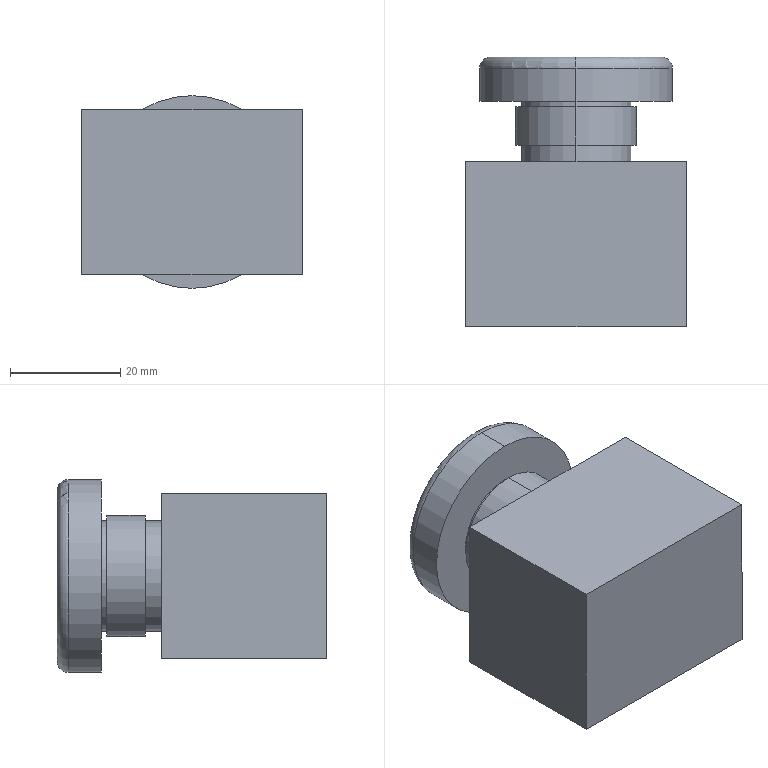Part | SolidWorks | features Boss 3, Cut 1, Extrusion 1, Fillet 1, LibraryFeature 1 | 1 solid | 20 faces | box 40 x 49 x 35 mm | volume 47522 mm3 | plane 10 | cylinder 8 | torus 2 | commonest cylinder face diameters 20 x4 22 x2 35 x2
STEP:
#1=CARTESIAN_POINT('',(0.,15.,10.));
#2=VERTEX_POINT('',#1);
#3=CARTESIAN_POINT('',(0.,15.,-10.));
#4=VERTEX_POINT('',#3);
#5=CARTESIAN_POINT('',(0.,15.,0.));
#6=DIRECTION('',(0.,1.,0.));
#7=DIRECTION('',(0.,0.,1.));
#8=AXIS2_PLACEMENT_3D('',#5,#6,#7);
#9=CIRCLE('',#8,10.);
#10=EDGE_CURVE('',#2,#4,#9,.T.);
#11=ORIENTED_EDGE('',*,*,#10,.T.);
#12=CARTESIAN_POINT('',(0.,18.,-10.));
#13=VERTEX_POINT('',#12);
#14=CARTESIAN_POINT('',(0.,15.,-10.));
#15=DIRECTION('',(0.,1.,0.));
#16=VECTOR('',#15,1000.);
#17=LINE('',#14,#16);
#18=EDGE_CURVE('',#4,#13,#17,.T.);
#19=ORIENTED_EDGE('',*,*,#18,.T.);
#20=CARTESIAN_POINT('',(0.,18.,10.));
#21=VERTEX_POINT('',#20);
#22=CARTESIAN_POINT('',(0.,18.,0.));
#23=DIRECTION('',(0.,1.,0.));
#24=DIRECTION('',(0.,0.,1.));
#25=AXIS2_PLACEMENT_3D('',#22,#23,#24);
#26=CIRCLE('',#25,10.);
#27=EDGE_CURVE('',#21,#13,#26,.T.);
#28=ORIENTED_EDGE('',*,*,#27,.F.);
#29=CARTESIAN_POINT('',(0.,15.,10.));
#30=DIRECTION('',(0.,1.,0.));
#31=VECTOR('',#30,1000.);
#32=LINE('',#29,#31);
#33=EDGE_CURVE('',#2,#21,#32,.T.);
#34=ORIENTED_EDGE('',*,*,#33,.F.);
#35=EDGE_LOOP('',(#11,#19,#28,#34));
#36=FACE_OUTER_BOUND('',#35,.T.);
#37=CARTESIAN_POINT('',(0.,15.,0.));
#38=DIRECTION('',(0.,1.,0.));
#39=DIRECTION('',(0.,0.,1.));
#40=AXIS2_PLACEMENT_3D('',#37,#38,#39);
#41=CYLINDRICAL_SURFACE('',#40,10.);
#42=ADVANCED_FACE('',(#36),#41,.T.);
#43=CARTESIAN_POINT('',(0.,32.,-17.5));
#44=VERTEX_POINT('',#43);
#45=CARTESIAN_POINT('',(0.,32.,17.5));
#46=VERTEX_POINT('',#45);
#47=CARTESIAN_POINT('',(0.,32.,0.));
#48=DIRECTION('',(0.,-1.,0.));
#49=DIRECTION('',(0.,0.,1.));
#50=AXIS2_PLACEMENT_3D('',#47,#48,#49);
#51=CIRCLE('',#50,17.5);
#52=EDGE_CURVE('',#44,#46,#51,.T.);
#53=ORIENTED_EDGE('',*,*,#52,.F.);
#54=CARTESIAN_POINT('',(0.,34.,-15.5));
#55=VERTEX_POINT('',#54);
#56=CARTESIAN_POINT('',(0.,32.,-15.5));
#57=DIRECTION('',(1.,0.,0.));
#58=DIRECTION('',(0.,0.,-1.));
#59=AXIS2_PLACEMENT_3D('',#56,#57,#58);
#60=CIRCLE('',#59,2.);
#61=EDGE_CURVE('',#44,#55,#60,.T.);
#62=ORIENTED_EDGE('',*,*,#61,.T.);
#63=CARTESIAN_POINT('',(0.,34.,15.5));
#64=VERTEX_POINT('',#63);
#65=CARTESIAN_POINT('',(0.,34.,0.));
#66=DIRECTION('',(0.,1.,0.));
#67=DIRECTION('',(0.,0.,1.));
#68=AXIS2_PLACEMENT_3D('',#65,#66,#67);
#69=CIRCLE('',#68,15.5);
#70=EDGE_CURVE('',#64,#55,#69,.T.);
#71=ORIENTED_EDGE('',*,*,#70,.F.);
#72=CARTESIAN_POINT('',(0.,32.,15.5));
#73=DIRECTION('',(-1.,0.,0.));
#74=DIRECTION('',(0.,0.,1.));
#75=AXIS2_PLACEMENT_3D('',#72,#73,#74);
#76=CIRCLE('',#75,2.);
#77=EDGE_CURVE('',#46,#64,#76,.T.);
#78=ORIENTED_EDGE('',*,*,#77,.F.);
#79=EDGE_LOOP('',(#53,#62,#71,#78));
#80=FACE_OUTER_BOUND('',#79,.T.);
#81=CARTESIAN_POINT('',(0.,32.,0.));
#82=DIRECTION('',(0.,1.,0.));
#83=DIRECTION('',(0.,0.,1.));
#84=AXIS2_PLACEMENT_3D('',#81,#82,#83);
#85=TOROIDAL_SURFACE('',#84,15.5,2.);
#86=ADVANCED_FACE('',(#80),#85,.T.);
#87=ORIENTED_EDGE('',*,*,#52,.T.);
#88=CARTESIAN_POINT('',(0.,26.,17.5));
#89=VERTEX_POINT('',#88);
#90=CARTESIAN_POINT('',(0.,34.,17.5));
#91=DIRECTION('',(0.,-1.,0.));
#92=VECTOR('',#91,1000.);
#93=LINE('',#90,#92);
#94=EDGE_CURVE('',#46,#89,#93,.T.);
#95=ORIENTED_EDGE('',*,*,#94,.T.);
#96=CARTESIAN_POINT('',(0.,26.,-17.5));
#97=VERTEX_POINT('',#96);
#98=CARTESIAN_POINT('',(0.,26.,0.));
#99=DIRECTION('',(0.,1.,0.));
#100=DIRECTION('',(0.,0.,1.));
#101=AXIS2_PLACEMENT_3D('',#98,#99,#100);
#102=CIRCLE('',#101,17.5);
#103=EDGE_CURVE('',#89,#97,#102,.T.);
#104=ORIENTED_EDGE('',*,*,#103,.T.);
#105=CARTESIAN_POINT('',(0.,34.,-17.5));
#106=DIRECTION('',(0.,-1.,0.));
#107=VECTOR('',#106,1000.);
#108=LINE('',#105,#107);
#109=EDGE_CURVE('',#44,#97,#108,.T.);
#110=ORIENTED_EDGE('',*,*,#109,.F.);
#111=EDGE_LOOP('',(#87,#95,#104,#110));
#112=FACE_OUTER_BOUND('',#111,.T.);
#113=CARTESIAN_POINT('',(0.,34.,0.));
#114=DIRECTION('',(0.,-1.,0.));
#115=DIRECTION('',(0.,0.,-1.));
#116=AXIS2_PLACEMENT_3D('',#113,#114,#115);
#117=CYLINDRICAL_SURFACE('',#116,17.5);
#118=ADVANCED_FACE('',(#112),#117,.T.);
#119=CARTESIAN_POINT('',(0.,26.,10.));
#120=VERTEX_POINT('',#119);
#121=CARTESIAN_POINT('',(0.,26.,-10.));
#122=VERTEX_POINT('',#121);
#123=CARTESIAN_POINT('',(0.,26.,0.));
#124=DIRECTION('',(0.,1.,0.));
#125=DIRECTION('',(0.,0.,1.));
#126=AXIS2_PLACEMENT_3D('',#123,#124,#125);
#127=CIRCLE('',#126,10.);
#128=EDGE_CURVE('',#120,#122,#127,.T.);
#129=ORIENTED_EDGE('',*,*,#128,.F.);
#130=CARTESIAN_POINT('',(0.,25.,10.));
#131=VERTEX_POINT('',#130);
#132=CARTESIAN_POINT('',(0.,26.,10.));
#133=DIRECTION('',(0.,-1.,0.));
#134=VECTOR('',#133,1000.);
#135=LINE('',#132,#134);
#136=EDGE_CURVE('',#120,#131,#135,.T.);
#137=ORIENTED_EDGE('',*,*,#136,.T.);
#138=CARTESIAN_POINT('',(0.,25.,-10.));
#139=VERTEX_POINT('',#138);
#140=CARTESIAN_POINT('',(0.,25.,0.));
#141=DIRECTION('',(0.,1.,0.));
#142=DIRECTION('',(0.,0.,1.));
#143=AXIS2_PLACEMENT_3D('',#140,#141,#142);
#144=CIRCLE('',#143,10.);
#145=EDGE_CURVE('',#131,#139,#144,.T.);
#146=ORIENTED_EDGE('',*,*,#145,.T.);
#147=CARTESIAN_POINT('',(0.,26.,-10.));
#148=DIRECTION('',(0.,-1.,0.));
#149=VECTOR('',#148,1000.);
#150=LINE('',#147,#149);
#151=EDGE_CURVE('',#122,#139,#150,.T.);
#152=ORIENTED_EDGE('',*,*,#151,.F.);
#153=EDGE_LOOP('',(#129,#137,#146,#152));
#154=FACE_OUTER_BOUND('',#153,.T.);
#155=CARTESIAN_POINT('',(0.,26.,0.));
#156=DIRECTION('',(0.,-1.,0.));
#157=DIRECTION('',(0.,0.,-1.));
#158=AXIS2_PLACEMENT_3D('',#155,#156,#157);
#159=CYLINDRICAL_SURFACE('',#158,10.);
#160=ADVANCED_FACE('',(#154),#159,.T.);
#161=CARTESIAN_POINT('',(0.,25.,11.));
#162=VERTEX_POINT('',#161);
#163=CARTESIAN_POINT('',(0.,25.,-11.));
#164=VERTEX_POINT('',#163);
#165=CARTESIAN_POINT('',(0.,25.,0.));
#166=DIRECTION('',(0.,1.,0.));
#167=DIRECTION('',(0.,0.,1.));
#168=AXIS2_PLACEMENT_3D('',#165,#166,#167);
#169=CIRCLE('',#168,11.);
#170=EDGE_CURVE('',#162,#164,#169,.T.);
#171=ORIENTED_EDGE('',*,*,#170,.F.);
#172=CARTESIAN_POINT('',(0.,18.,11.));
#173=VERTEX_POINT('',#172);
#174=CARTESIAN_POINT('',(0.,25.,11.));
#175=DIRECTION('',(0.,-1.,0.));
#176=VECTOR('',#175,1000.);
#177=LINE('',#174,#176);
#178=EDGE_CURVE('',#162,#173,#177,.T.);
#179=ORIENTED_EDGE('',*,*,#178,.T.);
#180=CARTESIAN_POINT('',(0.,18.,-11.));
#181=VERTEX_POINT('',#180);
#182=CARTESIAN_POINT('',(0.,18.,0.));
#183=DIRECTION('',(0.,1.,0.));
#184=DIRECTION('',(0.,0.,1.));
#185=AXIS2_PLACEMENT_3D('',#182,#183,#184);
#186=CIRCLE('',#185,11.);
#187=EDGE_CURVE('',#173,#181,#186,.T.);
#188=ORIENTED_EDGE('',*,*,#187,.T.);
#189=CARTESIAN_POINT('',(0.,25.,-11.));
#190=DIRECTION('',(0.,-1.,0.));
#191=VECTOR('',#190,1000.);
#192=LINE('',#189,#191);
#193=EDGE_CURVE('',#164,#181,#192,.T.);
#194=ORIENTED_EDGE('',*,*,#193,.F.);
#195=EDGE_LOOP('',(#171,#179,#188,#194));
#196=FACE_OUTER_BOUND('',#195,.T.);
#197=CARTESIAN_POINT('',(0.,25.,0.));
#198=DIRECTION('',(0.,-1.,0.));
#199=DIRECTION('',(0.,0.,-1.));
#200=AXIS2_PLACEMENT_3D('',#197,#198,#199);
#201=CYLINDRICAL_SURFACE('',#200,11.);
#202=ADVANCED_FACE('',(#196),#201,.T.);
#203=CARTESIAN_POINT('',(0.,25.,0.));
#204=DIRECTION('',(0.,1.,0.));
#205=DIRECTION('',(0.,0.,1.));
#206=AXIS2_PLACEMENT_3D('',#203,#204,#205);
#207=CIRCLE('',#206,11.);
#208=EDGE_CURVE('',#164,#162,#207,.T.);
#209=ORIENTED_EDGE('',*,*,#208,.T.);
#210=ORIENTED_EDGE('',*,*,#170,.T.);
#211=EDGE_LOOP('',(#209,#210));
#212=FACE_OUTER_BOUND('',#211,.T.);
#213=CARTESIAN_POINT('',(0.,25.,0.));
#214=DIRECTION('',(0.,1.,0.));
#215=DIRECTION('',(0.,0.,1.));
#216=AXIS2_PLACEMENT_3D('',#213,#214,#215);
#217=CIRCLE('',#216,10.);
#218=EDGE_CURVE('',#139,#131,#217,.T.);
#219=ORIENTED_EDGE('',*,*,#218,.F.);
#220=ORIENTED_EDGE('',*,*,#145,.F.);
#221=EDGE_LOOP('',(#219,#220));
#222=FACE_BOUND('',#221,.T.);
#223=CARTESIAN_POINT('',(0.,25.,0.));
#224=DIRECTION('',(0.,1.,0.));
#225=DIRECTION('',(0.,0.,1.));
#226=AXIS2_PLACEMENT_3D('',#223,#224,#225);
#227=PLANE('',#226);
#228=ADVANCED_FACE('',(#212,#222),#227,.T.);
#229=ORIENTED_EDGE('',*,*,#178,.F.);
#230=ORIENTED_EDGE('',*,*,#208,.F.);
#231=ORIENTED_EDGE('',*,*,#193,.T.);
#232=CARTESIAN_POINT('',(0.,18.,0.));
#233=DIRECTION('',(0.,1.,0.));
#234=DIRECTION('',(0.,0.,1.));
#235=AXIS2_PLACEMENT_3D('',#232,#233,#234);
#236=CIRCLE('',#235,11.);
#237=EDGE_CURVE('',#181,#173,#236,.T.);
#238=ORIENTED_EDGE('',*,*,#237,.T.);
#239=EDGE_LOOP('',(#229,#230,#231,#238));
#240=FACE_OUTER_BOUND('',#239,.T.);
#241=CARTESIAN_POINT('',(0.,25.,0.));
#242=DIRECTION('',(0.,-1.,0.));
#243=DIRECTION('',(0.,0.,-1.));
#244=AXIS2_PLACEMENT_3D('',#241,#242,#243);
#245=CYLINDRICAL_SURFACE('',#244,11.);
#246=ADVANCED_FACE('',(#240),#245,.T.);
#247=ORIENTED_EDGE('',*,*,#136,.F.);
#248=CARTESIAN_POINT('',(0.,26.,0.));
#249=DIRECTION('',(0.,1.,0.));
#250=DIRECTION('',(0.,0.,1.));
#251=AXIS2_PLACEMENT_3D('',#248,#249,#250);
#252=CIRCLE('',#251,10.);
#253=EDGE_CURVE('',#122,#120,#252,.T.);
#254=ORIENTED_EDGE('',*,*,#253,.F.);
#255=ORIENTED_EDGE('',*,*,#151,.T.);
#256=ORIENTED_EDGE('',*,*,#218,.T.);
#257=EDGE_LOOP('',(#247,#254,#255,#256));
#258=FACE_OUTER_BOUND('',#257,.T.);
#259=CARTESIAN_POINT('',(0.,26.,0.));
#260=DIRECTION('',(0.,-1.,0.));
#261=DIRECTION('',(0.,0.,-1.));
#262=AXIS2_PLACEMENT_3D('',#259,#260,#261);
#263=CYLINDRICAL_SURFACE('',#262,10.);
#264=ADVANCED_FACE('',(#258),#263,.T.);
#265=CARTESIAN_POINT('',(0.,26.,0.));
#266=DIRECTION('',(0.,1.,0.));
#267=DIRECTION('',(0.,0.,1.));
#268=AXIS2_PLACEMENT_3D('',#265,#266,#267);
#269=CIRCLE('',#268,17.5);
#270=EDGE_CURVE('',#97,#89,#269,.T.);
#271=ORIENTED_EDGE('',*,*,#270,.F.);
#272=ORIENTED_EDGE('',*,*,#103,.F.);
#273=EDGE_LOOP('',(#271,#272));
#274=FACE_OUTER_BOUND('',#273,.T.);
#275=ORIENTED_EDGE('',*,*,#253,.T.);
#276=ORIENTED_EDGE('',*,*,#128,.T.);
#277=EDGE_LOOP('',(#275,#276));
#278=FACE_BOUND('',#277,.T.);
#279=CARTESIAN_POINT('',(0.,26.,0.));
#280=DIRECTION('',(0.,1.,0.));
#281=DIRECTION('',(0.,0.,1.));
#282=AXIS2_PLACEMENT_3D('',#279,#280,#281);
#283=PLANE('',#282);
#284=ADVANCED_FACE('',(#274,#278),#283,.F.);
#285=ORIENTED_EDGE('',*,*,#94,.F.);
#286=CARTESIAN_POINT('',(0.,32.,0.));
#287=DIRECTION('',(0.,-1.,0.));
#288=DIRECTION('',(0.,0.,1.));
#289=AXIS2_PLACEMENT_3D('',#286,#287,#288);
#290=CIRCLE('',#289,17.5);
#291=EDGE_CURVE('',#46,#44,#290,.T.);
#292=ORIENTED_EDGE('',*,*,#291,.T.);
#293=ORIENTED_EDGE('',*,*,#109,.T.);
#294=ORIENTED_EDGE('',*,*,#270,.T.);
#295=EDGE_LOOP('',(#285,#292,#293,#294));
#296=FACE_OUTER_BOUND('',#295,.T.);
#297=CARTESIAN_POINT('',(0.,34.,0.));
#298=DIRECTION('',(0.,-1.,0.));
#299=DIRECTION('',(0.,0.,-1.));
#300=AXIS2_PLACEMENT_3D('',#297,#298,#299);
#301=CYLINDRICAL_SURFACE('',#300,17.5);
#302=ADVANCED_FACE('',(#296),#301,.T.);
#303=ORIENTED_EDGE('',*,*,#70,.T.);
#304=CARTESIAN_POINT('',(0.,34.,0.));
#305=DIRECTION('',(0.,1.,0.));
#306=DIRECTION('',(0.,0.,1.));
#307=AXIS2_PLACEMENT_3D('',#304,#305,#306);
#308=CIRCLE('',#307,15.5);
#309=EDGE_CURVE('',#55,#64,#308,.T.);
#310=ORIENTED_EDGE('',*,*,#309,.T.);
#311=EDGE_LOOP('',(#303,#310));
#312=FACE_OUTER_BOUND('',#311,.T.);
#313=CARTESIAN_POINT('',(0.,34.,0.));
#314=DIRECTION('',(0.,1.,0.));
#315=DIRECTION('',(0.,0.,1.));
#316=AXIS2_PLACEMENT_3D('',#313,#314,#315);
#317=PLANE('',#316);
#318=ADVANCED_FACE('',(#312),#317,.T.);
#319=ORIENTED_EDGE('',*,*,#61,.F.);
#320=ORIENTED_EDGE('',*,*,#291,.F.);
#321=ORIENTED_EDGE('',*,*,#77,.T.);
#322=ORIENTED_EDGE('',*,*,#309,.F.);
#323=EDGE_LOOP('',(#319,#320,#321,#322));
#324=FACE_OUTER_BOUND('',#323,.T.);
#325=CARTESIAN_POINT('',(0.,32.,0.));
#326=DIRECTION('',(0.,1.,0.));
#327=DIRECTION('',(0.,0.,1.));
#328=AXIS2_PLACEMENT_3D('',#325,#326,#327);
#329=TOROIDAL_SURFACE('',#328,15.5,2.);
#330=ADVANCED_FACE('',(#324),#329,.T.);
#331=ORIENTED_EDGE('',*,*,#27,.T.);
#332=CARTESIAN_POINT('',(0.,18.,0.));
#333=DIRECTION('',(0.,1.,0.));
#334=DIRECTION('',(0.,0.,1.));
#335=AXIS2_PLACEMENT_3D('',#332,#333,#334);
#336=CIRCLE('',#335,10.);
#337=EDGE_CURVE('',#13,#21,#336,.T.);
#338=ORIENTED_EDGE('',*,*,#337,.T.);
#339=EDGE_LOOP('',(#331,#338));
#340=FACE_BOUND('',#339,.T.);
#341=ORIENTED_EDGE('',*,*,#237,.F.);
#342=ORIENTED_EDGE('',*,*,#187,.F.);
#343=EDGE_LOOP('',(#341,#342));
#344=FACE_OUTER_BOUND('',#343,.T.);
#345=CARTESIAN_POINT('',(0.,18.,0.));
#346=DIRECTION('',(0.,1.,0.));
#347=DIRECTION('',(0.,0.,1.));
#348=AXIS2_PLACEMENT_3D('',#345,#346,#347);
#349=PLANE('',#348);
#350=ADVANCED_FACE('',(#340,#344),#349,.F.);
#351=ORIENTED_EDGE('',*,*,#18,.F.);
#352=CARTESIAN_POINT('',(0.,15.,0.));
#353=DIRECTION('',(0.,1.,0.));
#354=DIRECTION('',(0.,0.,1.));
#355=AXIS2_PLACEMENT_3D('',#352,#353,#354);
#356=CIRCLE('',#355,10.);
#357=EDGE_CURVE('',#4,#2,#356,.T.);
#358=ORIENTED_EDGE('',*,*,#357,.T.);
#359=ORIENTED_EDGE('',*,*,#33,.T.);
#360=ORIENTED_EDGE('',*,*,#337,.F.);
#361=EDGE_LOOP('',(#351,#358,#359,#360));
#362=FACE_OUTER_BOUND('',#361,.T.);
#363=CARTESIAN_POINT('',(0.,15.,0.));
#364=DIRECTION('',(0.,1.,0.));
#365=DIRECTION('',(0.,0.,1.));
#366=AXIS2_PLACEMENT_3D('',#363,#364,#365);
#367=CYLINDRICAL_SURFACE('',#366,10.);
#368=ADVANCED_FACE('',(#362),#367,.T.);
#369=CARTESIAN_POINT('',(-20.,-15.,-15.));
#370=VERTEX_POINT('',#369);
#371=CARTESIAN_POINT('',(-20.,-15.,15.));
#372=VERTEX_POINT('',#371);
#373=CARTESIAN_POINT('',(-20.,-15.,-15.));
#374=DIRECTION('',(0.,0.,1.));
#375=VECTOR('',#374,1000.);
#376=LINE('',#373,#375);
#377=EDGE_CURVE('',#370,#372,#376,.T.);
#378=ORIENTED_EDGE('',*,*,#377,.F.);
#379=CARTESIAN_POINT('',(20.,-15.,-15.));
#380=VERTEX_POINT('',#379);
#381=CARTESIAN_POINT('',(-20.,-15.,-15.));
#382=DIRECTION('',(-1.,0.,0.));
#383=VECTOR('',#382,1000.);
#384=LINE('',#381,#383);
#385=EDGE_CURVE('',#380,#370,#384,.T.);
#386=ORIENTED_EDGE('',*,*,#385,.F.);
#387=CARTESIAN_POINT('',(20.,-15.,15.));
#388=VERTEX_POINT('',#387);
#389=CARTESIAN_POINT('',(20.,-15.,-15.));
#390=DIRECTION('',(0.,0.,-1.));
#391=VECTOR('',#390,1000.);
#392=LINE('',#389,#391);
#393=EDGE_CURVE('',#388,#380,#392,.T.);
#394=ORIENTED_EDGE('',*,*,#393,.F.);
#395=CARTESIAN_POINT('',(-20.,-15.,15.));
#396=DIRECTION('',(1.,0.,0.));
#397=VECTOR('',#396,1000.);
#398=LINE('',#395,#397);
#399=EDGE_CURVE('',#372,#388,#398,.T.);
#400=ORIENTED_EDGE('',*,*,#399,.F.);
#401=EDGE_LOOP('',(#378,#386,#394,#400));
#402=FACE_OUTER_BOUND('',#401,.T.);
#403=CARTESIAN_POINT('',(-20.,-15.,-15.));
#404=DIRECTION('',(0.,1.,0.));
#405=DIRECTION('',(0.,0.,1.));
#406=AXIS2_PLACEMENT_3D('',#403,#404,#405);
#407=PLANE('',#406);
#408=ADVANCED_FACE('',(#402),#407,.F.);
#409=ORIENTED_EDGE('',*,*,#385,.T.);
#410=CARTESIAN_POINT('',(-20.,15.,-15.));
#411=VERTEX_POINT('',#410);
#412=CARTESIAN_POINT('',(-20.,15.,-15.));
#413=DIRECTION('',(0.,-1.,0.));
#414=VECTOR('',#413,1000.);
#415=LINE('',#412,#414);
#416=EDGE_CURVE('',#411,#370,#415,.T.);
#417=ORIENTED_EDGE('',*,*,#416,.F.);
#418=CARTESIAN_POINT('',(20.,15.,-15.));
#419=VERTEX_POINT('',#418);
#420=CARTESIAN_POINT('',(-20.,15.,-15.));
#421=DIRECTION('',(-1.,0.,0.));
#422=VECTOR('',#421,1000.);
#423=LINE('',#420,#422);
#424=EDGE_CURVE('',#419,#411,#423,.T.);
#425=ORIENTED_EDGE('',*,*,#424,.F.);
#426=CARTESIAN_POINT('',(20.,15.,-15.));
#427=DIRECTION('',(0.,-1.,0.));
#428=VECTOR('',#427,1000.);
#429=LINE('',#426,#428);
#430=EDGE_CURVE('',#419,#380,#429,.T.);
#431=ORIENTED_EDGE('',*,*,#430,.T.);
#432=EDGE_LOOP('',(#409,#417,#425,#431));
#433=FACE_OUTER_BOUND('',#432,.T.);
#434=CARTESIAN_POINT('',(-20.,15.,-15.));
#435=DIRECTION('',(0.,0.,1.));
#436=DIRECTION('',(1.,0.,0.));
#437=AXIS2_PLACEMENT_3D('',#434,#435,#436);
#438=PLANE('',#437);
#439=ADVANCED_FACE('',(#433),#438,.F.);
#440=ORIENTED_EDGE('',*,*,#393,.T.);
#441=ORIENTED_EDGE('',*,*,#430,.F.);
#442=CARTESIAN_POINT('',(20.,15.,15.));
#443=VERTEX_POINT('',#442);
#444=CARTESIAN_POINT('',(20.,15.,-15.));
#445=DIRECTION('',(0.,0.,-1.));
#446=VECTOR('',#445,1000.);
#447=LINE('',#444,#446);
#448=EDGE_CURVE('',#443,#419,#447,.T.);
#449=ORIENTED_EDGE('',*,*,#448,.F.);
#450=CARTESIAN_POINT('',(20.,15.,15.));
#451=DIRECTION('',(0.,-1.,0.));
#452=VECTOR('',#451,1000.);
#453=LINE('',#450,#452);
#454=EDGE_CURVE('',#443,#388,#453,.T.);
#455=ORIENTED_EDGE('',*,*,#454,.T.);
#456=EDGE_LOOP('',(#440,#441,#449,#455));
#457=FACE_OUTER_BOUND('',#456,.T.);
#458=CARTESIAN_POINT('',(20.,15.,-15.));
#459=DIRECTION('',(-1.,0.,0.));
#460=DIRECTION('',(0.,0.,1.));
#461=AXIS2_PLACEMENT_3D('',#458,#459,#460);
#462=PLANE('',#461);
#463=ADVANCED_FACE('',(#457),#462,.F.);
#464=ORIENTED_EDGE('',*,*,#399,.T.);
#465=ORIENTED_EDGE('',*,*,#454,.F.);
#466=CARTESIAN_POINT('',(-20.,15.,15.));
#467=VERTEX_POINT('',#466);
#468=CARTESIAN_POINT('',(-20.,15.,15.));
#469=DIRECTION('',(1.,0.,0.));
#470=VECTOR('',#469,1000.);
#471=LINE('',#468,#470);
#472=EDGE_CURVE('',#467,#443,#471,.T.);
#473=ORIENTED_EDGE('',*,*,#472,.F.);
#474=CARTESIAN_POINT('',(-20.,15.,15.));
#475=DIRECTION('',(0.,-1.,0.));
#476=VECTOR('',#475,1000.);
#477=LINE('',#474,#476);
#478=EDGE_CURVE('',#467,#372,#477,.T.);
#479=ORIENTED_EDGE('',*,*,#478,.T.);
#480=EDGE_LOOP('',(#464,#465,#473,#479));
#481=FACE_OUTER_BOUND('',#480,.T.);
#482=CARTESIAN_POINT('',(-20.,15.,15.));
#483=DIRECTION('',(0.,0.,-1.));
#484=DIRECTION('',(-1.,0.,0.));
#485=AXIS2_PLACEMENT_3D('',#482,#483,#484);
#486=PLANE('',#485);
#487=ADVANCED_FACE('',(#481),#486,.F.);
#488=ORIENTED_EDGE('',*,*,#377,.T.);
#489=ORIENTED_EDGE('',*,*,#478,.F.);
#490=CARTESIAN_POINT('',(-20.,15.,-15.));
#491=DIRECTION('',(0.,0.,1.));
#492=VECTOR('',#491,1000.);
#493=LINE('',#490,#492);
#494=EDGE_CURVE('',#411,#467,#493,.T.);
#495=ORIENTED_EDGE('',*,*,#494,.F.);
#496=ORIENTED_EDGE('',*,*,#416,.T.);
#497=EDGE_LOOP('',(#488,#489,#495,#496));
#498=FACE_OUTER_BOUND('',#497,.T.);
#499=CARTESIAN_POINT('',(-20.,15.,-15.));
#500=DIRECTION('',(1.,0.,0.));
#501=DIRECTION('',(0.,0.,-1.));
#502=AXIS2_PLACEMENT_3D('',#499,#500,#501);
#503=PLANE('',#502);
#504=ADVANCED_FACE('',(#498),#503,.F.);
#505=ORIENTED_EDGE('',*,*,#494,.T.);
#506=ORIENTED_EDGE('',*,*,#472,.T.);
#507=ORIENTED_EDGE('',*,*,#448,.T.);
#508=ORIENTED_EDGE('',*,*,#424,.T.);
#509=EDGE_LOOP('',(#505,#506,#507,#508));
#510=FACE_OUTER_BOUND('',#509,.T.);
#511=ORIENTED_EDGE('',*,*,#10,.F.);
#512=ORIENTED_EDGE('',*,*,#357,.F.);
#513=EDGE_LOOP('',(#511,#512));
#514=FACE_BOUND('',#513,.T.);
#515=CARTESIAN_POINT('',(-20.,15.,-15.));
#516=DIRECTION('',(0.,1.,0.));
#517=DIRECTION('',(0.,0.,1.));
#518=AXIS2_PLACEMENT_3D('',#515,#516,#517);
#519=PLANE('',#518);
#520=ADVANCED_FACE('',(#510,#514),#519,.T.);
#521=CLOSED_SHELL('',(#42,#86,#118,#160,#202,#228,#246,#264,#284,#302,#318,#330,#350,#368,#408,#439,#463,#487,#504,#520));
#522=MANIFOLD_SOLID_BREP('',#521);
#523=CARTESIAN_POINT('',(0.,0.,0.));
#524=DIRECTION('',(0.,0.,1.));
#525=DIRECTION('',(1.,0.,0.));
#526=AXIS2_PLACEMENT_3D('',#523,#524,#525);
#527=(LENGTH_UNIT()NAMED_UNIT(*)SI_UNIT(.MILLI.,.METRE.));
#528=UNCERTAINTY_MEASURE_WITH_UNIT(LENGTH_MEASURE(0.00001),#527,'','');
#529=(NAMED_UNIT(*)PLANE_ANGLE_UNIT()SI_UNIT($,.RADIAN.));
#530=(NAMED_UNIT(*)SI_UNIT($,.STERADIAN.)SOLID_ANGLE_UNIT());
#531=(GEOMETRIC_REPRESENTATION_CONTEXT(3)GLOBAL_UNCERTAINTY_ASSIGNED_CONTEXT((#528))GLOBAL_UNIT_ASSIGNED_CONTEXT((#527,#529,#530))REPRESENTATION_CONTEXT('',''));
#532=ADVANCED_BREP_SHAPE_REPRESENTATION('',(#522,#526),#531);